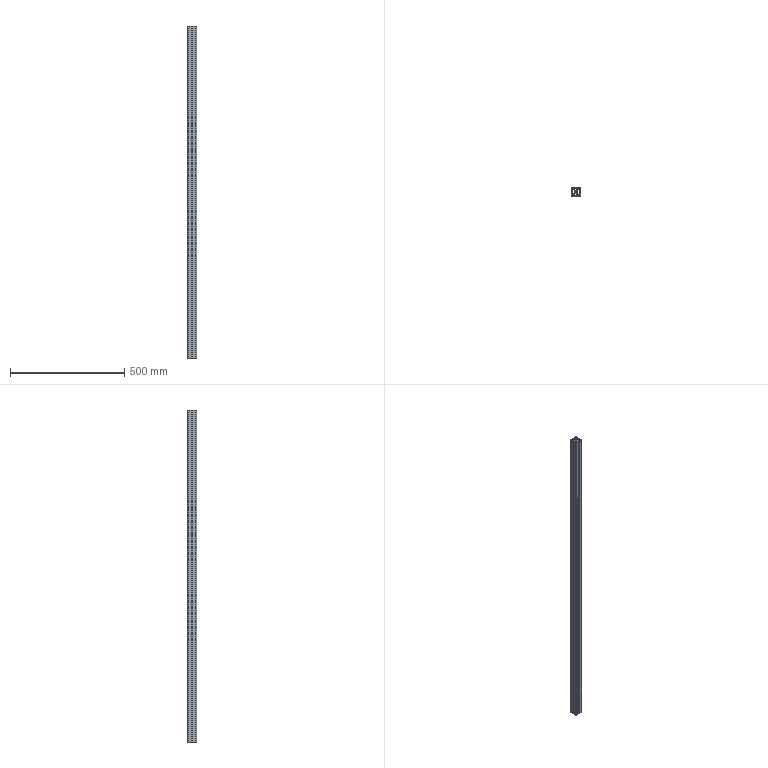Part | STEP file | 40x40-1450 | 1 solid | 88 faces | box 40 x 40 x 1450 mm | volume 1020723 mm3 | plane 78 | cylinder 10 | commonest cylinder face diameters 4 x4 10 x4 6.8 x2